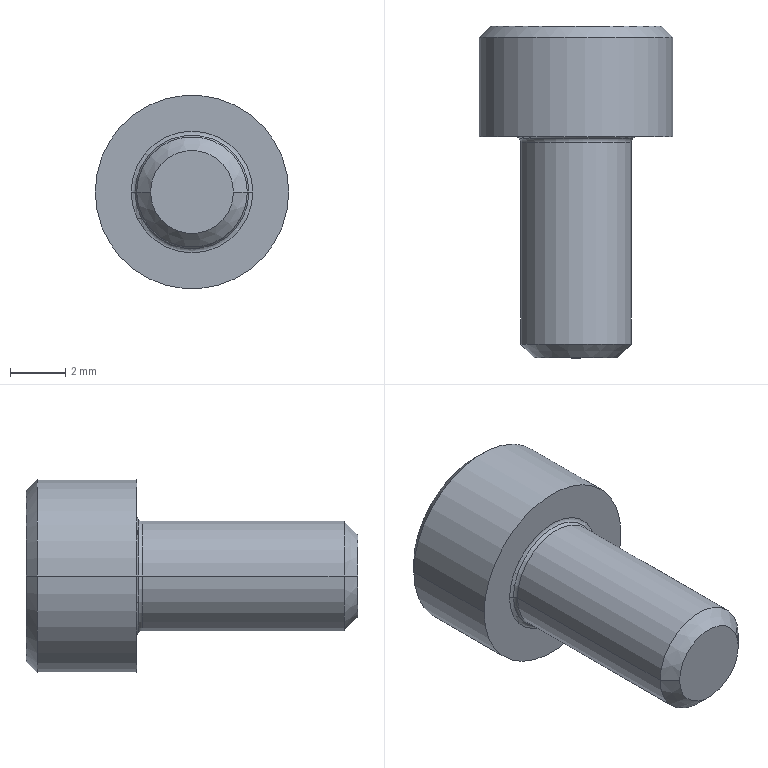Part | Creo | 1 solid | 23 faces | box 7 x 12 x 7 mm | volume 232.803 mm3 | plane 9 | cone 6 | cylinder 4 | torus 4 | commonest cylinder face diameters 4 x2 7 x2
STEP:
#1=CARTESIAN_POINT('',(-77.018,347.995,-340.));
#2=VERTEX_POINT('',#1);
#3=CARTESIAN_POINT('',(-77.884,347.995,-341.5));
#4=VERTEX_POINT('',#3);
#5=CARTESIAN_POINT('',(-77.018,347.995,-340.));
#6=CARTESIAN_POINT('',(-77.058,347.972,-340.07));
#7=CARTESIAN_POINT('',(-77.139,347.93,-340.21));
#8=CARTESIAN_POINT('',(-77.263,347.884,-340.425));
#9=CARTESIAN_POINT('',(-77.389,347.86,-340.642));
#10=CARTESIAN_POINT('',(-77.514,347.86,-340.859));
#11=CARTESIAN_POINT('',(-77.639,347.885,-341.076));
#12=CARTESIAN_POINT('',(-77.763,347.93,-341.291));
#13=CARTESIAN_POINT('',(-77.844,347.972,-341.431));
#14=CARTESIAN_POINT('',(-77.884,347.995,-341.5));
#15=B_SPLINE_CURVE_WITH_KNOTS('',3,(#5,#6,#7,#8,#9,#10,#11,#12,#13,#14),.UNSPECIFIED.,.F.,.F.,(4,1,1,1,1,1,1,4),(0.,0.1429,0.2857,0.4286,0.5714,0.7143,0.8571,1.),.UNSPECIFIED.);
#16=EDGE_CURVE('',#2,#4,#15,.T.);
#17=ORIENTED_EDGE('',*,*,#16,.F.);
#18=CARTESIAN_POINT('',(-78.75,346.995,-340.));
#19=VERTEX_POINT('',#18);
#20=CARTESIAN_POINT('',(-78.75,346.995,-340.));
#21=DIRECTION('',(0.866,0.5,0.));
#22=VECTOR('',#21,2.);
#23=LINE('',#20,#22);
#24=EDGE_CURVE('',#19,#2,#23,.T.);
#25=ORIENTED_EDGE('',*,*,#24,.F.);
#26=CARTESIAN_POINT('',(-80.482,347.995,-340.));
#27=VERTEX_POINT('',#26);
#28=CARTESIAN_POINT('',(-78.75,346.995,-340.));
#29=DIRECTION('',(-0.866,0.5,0.));
#30=VECTOR('',#29,2.);
#31=LINE('',#28,#30);
#32=EDGE_CURVE('',#19,#27,#31,.T.);
#33=ORIENTED_EDGE('',*,*,#32,.T.);
#34=CARTESIAN_POINT('',(-79.616,347.995,-341.5));
#35=VERTEX_POINT('',#34);
#36=CARTESIAN_POINT('',(-79.616,347.995,-341.5));
#37=CARTESIAN_POINT('',(-79.656,347.972,-341.43));
#38=CARTESIAN_POINT('',(-79.737,347.93,-341.29));
#39=CARTESIAN_POINT('',(-79.861,347.884,-341.075));
#40=CARTESIAN_POINT('',(-79.987,347.86,-340.858));
#41=CARTESIAN_POINT('',(-80.112,347.86,-340.641));
#42=CARTESIAN_POINT('',(-80.237,347.885,-340.424));
#43=CARTESIAN_POINT('',(-80.361,347.93,-340.209));
#44=CARTESIAN_POINT('',(-80.442,347.972,-340.069));
#45=CARTESIAN_POINT('',(-80.482,347.995,-340.));
#46=B_SPLINE_CURVE_WITH_KNOTS('',3,(#36,#37,#38,#39,#40,#41,#42,#43,#44,#45),.UNSPECIFIED.,.F.,.F.,(4,1,1,1,1,1,1,4),(0.,0.1429,0.2857,0.4286,0.5714,0.7143,0.8571,1.),.UNSPECIFIED.);
#47=EDGE_CURVE('',#35,#27,#46,.T.);
#48=ORIENTED_EDGE('',*,*,#47,.F.);
#49=CARTESIAN_POINT('',(-77.884,347.995,-341.5));
#50=CARTESIAN_POINT('',(-77.927,347.983,-341.5));
#51=CARTESIAN_POINT('',(-78.013,347.959,-341.5));
#52=CARTESIAN_POINT('',(-78.137,347.93,-341.5));
#53=CARTESIAN_POINT('',(-78.258,347.906,-341.5));
#54=CARTESIAN_POINT('',(-78.379,347.887,-341.5));
#55=CARTESIAN_POINT('',(-78.502,347.872,-341.5));
#56=CARTESIAN_POINT('',(-78.625,347.863,-341.5));
#57=CARTESIAN_POINT('',(-78.75,347.86,-341.5));
#58=CARTESIAN_POINT('',(-78.875,347.863,-341.5));
#59=CARTESIAN_POINT('',(-78.998,347.872,-341.5));
#60=CARTESIAN_POINT('',(-79.121,347.887,-341.5));
#61=CARTESIAN_POINT('',(-79.242,347.906,-341.5));
#62=CARTESIAN_POINT('',(-79.363,347.93,-341.5));
#63=CARTESIAN_POINT('',(-79.487,347.959,-341.5));
#64=CARTESIAN_POINT('',(-79.573,347.983,-341.5));
#65=CARTESIAN_POINT('',(-79.616,347.995,-341.5));
#66=B_SPLINE_CURVE_WITH_KNOTS('',3,(#49,#50,#51,#52,#53,#54,#55,#56,#57,#58,#59,#60,#61,#62,#63,#64,#65),.UNSPECIFIED.,.F.,.F.,(4,1,1,1,1,1,1,1,1,1,1,1,1,1,4),(0.,0.07143,0.1429,0.2143,0.2857,0.3571,0.4286,0.5,0.5714,0.6429,0.7143,0.7857,0.8571,0.9286,1.),.UNSPECIFIED.);
#67=EDGE_CURVE('',#4,#35,#66,.T.);
#68=ORIENTED_EDGE('',*,*,#67,.F.);
#69=EDGE_LOOP('',(#17,#25,#33,#48,#68));
#70=FACE_OUTER_BOUND('',#69,.F.);
#71=CARTESIAN_POINT('',(-78.75,347.505,-340.));
#72=DIRECTION('',(0.,1.,0.));
#73=DIRECTION('',(1.,0.,0.));
#74=AXIS2_PLACEMENT_3D('',#71,#72,#73);
#75=CONICAL_SURFACE('',#74,0.8833,60.);
#76=ADVANCED_FACE('',(#70),#75,.F.);
#77=CARTESIAN_POINT('',(-77.884,349.995,-341.5));
#78=VERTEX_POINT('',#77);
#79=CARTESIAN_POINT('',(-77.018,349.995,-340.));
#80=VERTEX_POINT('',#79);
#81=CARTESIAN_POINT('',(-77.884,349.995,-341.5));
#82=DIRECTION('',(0.5,0.,0.866));
#83=VECTOR('',#82,1.732);
#84=LINE('',#81,#83);
#85=EDGE_CURVE('',#78,#80,#84,.T.);
#86=ORIENTED_EDGE('',*,*,#85,.T.);
#87=CARTESIAN_POINT('',(-77.018,349.995,-340.));
#88=DIRECTION('',(0.,-1.,0.));
#89=VECTOR('',#88,2.);
#90=LINE('',#87,#89);
#91=EDGE_CURVE('',#80,#2,#90,.T.);
#92=ORIENTED_EDGE('',*,*,#91,.T.);
#93=ORIENTED_EDGE('',*,*,#16,.T.);
#94=CARTESIAN_POINT('',(-77.884,349.995,-341.5));
#95=DIRECTION('',(0.,-1.,0.));
#96=VECTOR('',#95,2.);
#97=LINE('',#94,#96);
#98=EDGE_CURVE('',#78,#4,#97,.T.);
#99=ORIENTED_EDGE('',*,*,#98,.F.);
#100=EDGE_LOOP('',(#86,#92,#93,#99));
#101=FACE_OUTER_BOUND('',#100,.F.);
#102=CARTESIAN_POINT('',(-77.884,347.995,-341.5));
#103=DIRECTION('',(-0.866,0.,0.5));
#104=DIRECTION('',(0.5,0.,0.866));
#105=AXIS2_PLACEMENT_3D('',#102,#103,#104);
#106=PLANE('',#105);
#107=ADVANCED_FACE('',(#101),#106,.T.);
#108=CARTESIAN_POINT('',(-75.65,349.995,-340.));
#109=VERTEX_POINT('',#108);
#110=CARTESIAN_POINT('',(-81.85,349.995,-340.));
#111=VERTEX_POINT('',#110);
#112=CARTESIAN_POINT('',(-78.75,349.995,-340.));
#113=DIRECTION('',(0.,1.,0.));
#114=DIRECTION('',(1.,0.,0.));
#115=AXIS2_PLACEMENT_3D('',#112,#113,#114);
#116=CIRCLE('',#115,3.1);
#117=EDGE_CURVE('',#109,#111,#116,.T.);
#118=ORIENTED_EDGE('',*,*,#117,.F.);
#119=CARTESIAN_POINT('',(-78.75,349.995,-340.));
#120=DIRECTION('',(0.,1.,0.));
#121=DIRECTION('',(-1.,0.,0.));
#122=AXIS2_PLACEMENT_3D('',#119,#120,#121);
#123=CIRCLE('',#122,3.1);
#124=EDGE_CURVE('',#111,#109,#123,.T.);
#125=ORIENTED_EDGE('',*,*,#124,.F.);
#126=EDGE_LOOP('',(#118,#125));
#127=FACE_OUTER_BOUND('',#126,.F.);
#128=CARTESIAN_POINT('',(-77.884,349.995,-338.5));
#129=VERTEX_POINT('',#128);
#130=CARTESIAN_POINT('',(-77.018,349.995,-340.));
#131=DIRECTION('',(-0.5,0.,0.866));
#132=VECTOR('',#131,1.732);
#133=LINE('',#130,#132);
#134=EDGE_CURVE('',#80,#129,#133,.T.);
#135=ORIENTED_EDGE('',*,*,#134,.F.);
#136=ORIENTED_EDGE('',*,*,#85,.F.);
#137=CARTESIAN_POINT('',(-79.616,349.995,-341.5));
#138=VERTEX_POINT('',#137);
#139=CARTESIAN_POINT('',(-77.884,349.995,-341.5));
#140=DIRECTION('',(-1.,0.,0.));
#141=VECTOR('',#140,1.732);
#142=LINE('',#139,#141);
#143=EDGE_CURVE('',#78,#138,#142,.T.);
#144=ORIENTED_EDGE('',*,*,#143,.T.);
#145=CARTESIAN_POINT('',(-80.482,349.995,-340.));
#146=VERTEX_POINT('',#145);
#147=CARTESIAN_POINT('',(-80.482,349.995,-340.));
#148=DIRECTION('',(0.5,0.,-0.866));
#149=VECTOR('',#148,1.732);
#150=LINE('',#147,#149);
#151=EDGE_CURVE('',#146,#138,#150,.T.);
#152=ORIENTED_EDGE('',*,*,#151,.F.);
#153=CARTESIAN_POINT('',(-79.616,349.995,-338.5));
#154=VERTEX_POINT('',#153);
#155=CARTESIAN_POINT('',(-79.616,349.995,-338.5));
#156=DIRECTION('',(-0.5,0.,-0.866));
#157=VECTOR('',#156,1.732);
#158=LINE('',#155,#157);
#159=EDGE_CURVE('',#154,#146,#158,.T.);
#160=ORIENTED_EDGE('',*,*,#159,.F.);
#161=CARTESIAN_POINT('',(-79.616,349.995,-338.5));
#162=DIRECTION('',(1.,0.,0.));
#163=VECTOR('',#162,1.732);
#164=LINE('',#161,#163);
#165=EDGE_CURVE('',#154,#129,#164,.T.);
#166=ORIENTED_EDGE('',*,*,#165,.T.);
#167=EDGE_LOOP('',(#135,#136,#144,#152,#160,#166));
#168=FACE_BOUND('',#167,.F.);
#169=CARTESIAN_POINT('',(-78.75,349.995,-340.));
#170=DIRECTION('',(0.,1.,0.));
#171=DIRECTION('',(1.,0.,0.));
#172=AXIS2_PLACEMENT_3D('',#169,#170,#171);
#173=PLANE('',#172);
#174=ADVANCED_FACE('',(#127,#168),#173,.T.);
#175=CARTESIAN_POINT('',(-75.25,349.595,-340.));
#176=VERTEX_POINT('',#175);
#177=CARTESIAN_POINT('',(-82.25,349.595,-340.));
#178=VERTEX_POINT('',#177);
#179=CARTESIAN_POINT('',(-78.75,349.595,-340.));
#180=DIRECTION('',(0.,1.,0.));
#181=DIRECTION('',(1.,0.,0.));
#182=AXIS2_PLACEMENT_3D('',#179,#180,#181);
#183=CIRCLE('',#182,3.5);
#184=EDGE_CURVE('',#176,#178,#183,.T.);
#185=ORIENTED_EDGE('',*,*,#184,.F.);
#186=CARTESIAN_POINT('',(-75.65,349.995,-340.));
#187=DIRECTION('',(0.7071,-0.7071,0.));
#188=VECTOR('',#187,0.5657);
#189=LINE('',#186,#188);
#190=EDGE_CURVE('',#109,#176,#189,.T.);
#191=ORIENTED_EDGE('',*,*,#190,.F.);
#192=ORIENTED_EDGE('',*,*,#117,.T.);
#193=CARTESIAN_POINT('',(-81.85,349.995,-340.));
#194=DIRECTION('',(-0.7071,-0.7071,0.));
#195=VECTOR('',#194,0.5657);
#196=LINE('',#193,#195);
#197=EDGE_CURVE('',#111,#178,#196,.T.);
#198=ORIENTED_EDGE('',*,*,#197,.T.);
#199=EDGE_LOOP('',(#185,#191,#192,#198));
#200=FACE_OUTER_BOUND('',#199,.F.);
#201=CARTESIAN_POINT('',(-78.75,349.795,-340.));
#202=DIRECTION('',(0.,-1.,0.));
#203=DIRECTION('',(-1.,0.,0.));
#204=AXIS2_PLACEMENT_3D('',#201,#202,#203);
#205=CONICAL_SURFACE('',#204,3.3,45.);
#206=ADVANCED_FACE('',(#200),#205,.T.);
#207=ORIENTED_EDGE('',*,*,#184,.T.);
#208=CARTESIAN_POINT('',(-82.25,345.995,-340.));
#209=VERTEX_POINT('',#208);
#210=CARTESIAN_POINT('',(-82.25,345.995,-340.));
#211=DIRECTION('',(0.,1.,0.));
#212=VECTOR('',#211,3.6);
#213=LINE('',#210,#212);
#214=EDGE_CURVE('',#209,#178,#213,.T.);
#215=ORIENTED_EDGE('',*,*,#214,.F.);
#216=CARTESIAN_POINT('',(-75.25,345.995,-340.));
#217=VERTEX_POINT('',#216);
#218=CARTESIAN_POINT('',(-78.75,345.995,-340.));
#219=DIRECTION('',(0.,-1.,0.));
#220=DIRECTION('',(-1.,0.,0.));
#221=AXIS2_PLACEMENT_3D('',#218,#219,#220);
#222=CIRCLE('',#221,3.5);
#223=EDGE_CURVE('',#209,#217,#222,.T.);
#224=ORIENTED_EDGE('',*,*,#223,.T.);
#225=CARTESIAN_POINT('',(-75.25,345.995,-340.));
#226=DIRECTION('',(0.,1.,0.));
#227=VECTOR('',#226,3.6);
#228=LINE('',#225,#227);
#229=EDGE_CURVE('',#217,#176,#228,.T.);
#230=ORIENTED_EDGE('',*,*,#229,.T.);
#231=EDGE_LOOP('',(#207,#215,#224,#230));
#232=FACE_OUTER_BOUND('',#231,.F.);
#233=CARTESIAN_POINT('',(-78.75,345.995,-340.));
#234=DIRECTION('',(0.,1.,0.));
#235=DIRECTION('',(1.,0.,0.));
#236=AXIS2_PLACEMENT_3D('',#233,#234,#235);
#237=CYLINDRICAL_SURFACE('',#236,3.5);
#238=ADVANCED_FACE('',(#232),#237,.T.);
#239=CARTESIAN_POINT('',(-78.75,349.595,-340.));
#240=DIRECTION('',(0.,1.,0.));
#241=DIRECTION('',(-1.,0.,0.));
#242=AXIS2_PLACEMENT_3D('',#239,#240,#241);
#243=CIRCLE('',#242,3.5);
#244=EDGE_CURVE('',#178,#176,#243,.T.);
#245=ORIENTED_EDGE('',*,*,#244,.T.);
#246=ORIENTED_EDGE('',*,*,#229,.F.);
#247=CARTESIAN_POINT('',(-78.75,345.995,-340.));
#248=DIRECTION('',(0.,-1.,0.));
#249=DIRECTION('',(1.,0.,0.));
#250=AXIS2_PLACEMENT_3D('',#247,#248,#249);
#251=CIRCLE('',#250,3.5);
#252=EDGE_CURVE('',#217,#209,#251,.T.);
#253=ORIENTED_EDGE('',*,*,#252,.T.);
#254=ORIENTED_EDGE('',*,*,#214,.T.);
#255=EDGE_LOOP('',(#245,#246,#253,#254));
#256=FACE_OUTER_BOUND('',#255,.F.);
#257=CARTESIAN_POINT('',(-78.75,345.995,-340.));
#258=DIRECTION('',(0.,1.,0.));
#259=DIRECTION('',(1.,0.,0.));
#260=AXIS2_PLACEMENT_3D('',#257,#258,#259);
#261=CYLINDRICAL_SURFACE('',#260,3.5);
#262=ADVANCED_FACE('',(#256),#261,.T.);
#263=ORIENTED_EDGE('',*,*,#244,.F.);
#264=ORIENTED_EDGE('',*,*,#197,.F.);
#265=ORIENTED_EDGE('',*,*,#124,.T.);
#266=ORIENTED_EDGE('',*,*,#190,.T.);
#267=EDGE_LOOP('',(#263,#264,#265,#266));
#268=FACE_OUTER_BOUND('',#267,.F.);
#269=CARTESIAN_POINT('',(-78.75,349.795,-340.));
#270=DIRECTION('',(0.,-1.,0.));
#271=DIRECTION('',(-1.,0.,0.));
#272=AXIS2_PLACEMENT_3D('',#269,#270,#271);
#273=CONICAL_SURFACE('',#272,3.3,45.);
#274=ADVANCED_FACE('',(#268),#273,.T.);
#275=ORIENTED_EDGE('',*,*,#252,.F.);
#276=ORIENTED_EDGE('',*,*,#223,.F.);
#277=EDGE_LOOP('',(#275,#276));
#278=FACE_OUTER_BOUND('',#277,.F.);
#279=CARTESIAN_POINT('',(-76.55,345.995,-340.));
#280=VERTEX_POINT('',#279);
#281=CARTESIAN_POINT('',(-80.95,345.995,-340.));
#282=VERTEX_POINT('',#281);
#283=CARTESIAN_POINT('',(-78.75,345.995,-340.));
#284=DIRECTION('',(0.,1.,0.));
#285=DIRECTION('',(1.,0.,0.));
#286=AXIS2_PLACEMENT_3D('',#283,#284,#285);
#287=CIRCLE('',#286,2.2);
#288=EDGE_CURVE('',#280,#282,#287,.T.);
#289=ORIENTED_EDGE('',*,*,#288,.F.);
#290=CARTESIAN_POINT('',(-78.75,345.995,-340.));
#291=DIRECTION('',(0.,1.,0.));
#292=DIRECTION('',(-1.,0.,0.));
#293=AXIS2_PLACEMENT_3D('',#290,#291,#292);
#294=CIRCLE('',#293,2.2);
#295=EDGE_CURVE('',#282,#280,#294,.T.);
#296=ORIENTED_EDGE('',*,*,#295,.F.);
#297=EDGE_LOOP('',(#289,#296));
#298=FACE_BOUND('',#297,.F.);
#299=CARTESIAN_POINT('',(-78.75,345.995,-340.));
#300=DIRECTION('',(0.,1.,0.));
#301=DIRECTION('',(1.,0.,0.));
#302=AXIS2_PLACEMENT_3D('',#299,#300,#301);
#303=PLANE('',#302);
#304=ADVANCED_FACE('',(#278,#298),#303,.F.);
#305=ORIENTED_EDGE('',*,*,#288,.T.);
#306=CARTESIAN_POINT('',(-80.809,345.937,-340.));
#307=VERTEX_POINT('',#306);
#308=CARTESIAN_POINT('',(-80.95,345.795,-340.));
#309=DIRECTION('',(0.,0.,-1.));
#310=DIRECTION('',(0.,1.,0.));
#311=AXIS2_PLACEMENT_3D('',#308,#309,#310);
#312=CIRCLE('',#311,0.2);
#313=EDGE_CURVE('',#282,#307,#312,.T.);
#314=ORIENTED_EDGE('',*,*,#313,.T.);
#315=CARTESIAN_POINT('',(-76.691,345.937,-340.));
#316=VERTEX_POINT('',#315);
#317=CARTESIAN_POINT('',(-78.75,345.937,-340.));
#318=DIRECTION('',(0.,1.,0.));
#319=DIRECTION('',(1.,0.,0.));
#320=AXIS2_PLACEMENT_3D('',#317,#318,#319);
#321=CIRCLE('',#320,2.059);
#322=EDGE_CURVE('',#316,#307,#321,.T.);
#323=ORIENTED_EDGE('',*,*,#322,.F.);
#324=CARTESIAN_POINT('',(-76.55,345.795,-340.));
#325=DIRECTION('',(0.,0.,1.));
#326=DIRECTION('',(0.,1.,0.));
#327=AXIS2_PLACEMENT_3D('',#324,#325,#326);
#328=CIRCLE('',#327,0.2);
#329=EDGE_CURVE('',#280,#316,#328,.T.);
#330=ORIENTED_EDGE('',*,*,#329,.F.);
#331=EDGE_LOOP('',(#305,#314,#323,#330));
#332=FACE_OUTER_BOUND('',#331,.F.);
#333=CARTESIAN_POINT('',(-78.75,345.795,-340.));
#334=DIRECTION('',(0.,1.,0.));
#335=DIRECTION('',(1.,0.,0.));
#336=AXIS2_PLACEMENT_3D('',#333,#334,#335);
#337=TOROIDAL_SURFACE('',#336,2.2,0.2);
#338=ADVANCED_FACE('',(#332),#337,.F.);
#339=ORIENTED_EDGE('',*,*,#295,.T.);
#340=ORIENTED_EDGE('',*,*,#329,.T.);
#341=CARTESIAN_POINT('',(-78.75,345.937,-340.));
#342=DIRECTION('',(0.,1.,0.));
#343=DIRECTION('',(-1.,0.,0.));
#344=AXIS2_PLACEMENT_3D('',#341,#342,#343);
#345=CIRCLE('',#344,2.059);
#346=EDGE_CURVE('',#307,#316,#345,.T.);
#347=ORIENTED_EDGE('',*,*,#346,.F.);
#348=ORIENTED_EDGE('',*,*,#313,.F.);
#349=EDGE_LOOP('',(#339,#340,#347,#348));
#350=FACE_OUTER_BOUND('',#349,.F.);
#351=CARTESIAN_POINT('',(-78.75,345.795,-340.));
#352=DIRECTION('',(0.,1.,0.));
#353=DIRECTION('',(1.,0.,0.));
#354=AXIS2_PLACEMENT_3D('',#351,#352,#353);
#355=TOROIDAL_SURFACE('',#354,2.2,0.2);
#356=ADVANCED_FACE('',(#350),#355,.F.);
#357=CARTESIAN_POINT('',(-80.75,345.795,-340.));
#358=VERTEX_POINT('',#357);
#359=CARTESIAN_POINT('',(-76.75,345.795,-340.));
#360=VERTEX_POINT('',#359);
#361=CARTESIAN_POINT('',(-78.75,345.795,-340.));
#362=DIRECTION('',(0.,1.,0.));
#363=DIRECTION('',(-1.,0.,0.));
#364=AXIS2_PLACEMENT_3D('',#361,#362,#363);
#365=CIRCLE('',#364,2.);
#366=EDGE_CURVE('',#358,#360,#365,.T.);
#367=ORIENTED_EDGE('',*,*,#366,.F.);
#368=CARTESIAN_POINT('',(-80.95,345.795,-340.));
#369=DIRECTION('',(0.,0.,-1.));
#370=DIRECTION('',(0.7071,0.7071,0.));
#371=AXIS2_PLACEMENT_3D('',#368,#369,#370);
#372=CIRCLE('',#371,0.2);
#373=EDGE_CURVE('',#307,#358,#372,.T.);
#374=ORIENTED_EDGE('',*,*,#373,.F.);
#375=ORIENTED_EDGE('',*,*,#346,.T.);
#376=CARTESIAN_POINT('',(-76.55,345.795,-340.));
#377=DIRECTION('',(0.,0.,1.));
#378=DIRECTION('',(-0.7071,0.7071,0.));
#379=AXIS2_PLACEMENT_3D('',#376,#377,#378);
#380=CIRCLE('',#379,0.2);
#381=EDGE_CURVE('',#316,#360,#380,.T.);
#382=ORIENTED_EDGE('',*,*,#381,.T.);
#383=EDGE_LOOP('',(#367,#374,#375,#382));
#384=FACE_OUTER_BOUND('',#383,.F.);
#385=CARTESIAN_POINT('',(-78.75,345.795,-340.));
#386=DIRECTION('',(0.,1.,0.));
#387=DIRECTION('',(1.,0.,0.));
#388=AXIS2_PLACEMENT_3D('',#385,#386,#387);
#389=TOROIDAL_SURFACE('',#388,2.2,0.2);
#390=ADVANCED_FACE('',(#384),#389,.F.);
#391=CARTESIAN_POINT('',(-76.75,338.495,-340.));
#392=VERTEX_POINT('',#391);
#393=CARTESIAN_POINT('',(-80.75,338.495,-340.));
#394=VERTEX_POINT('',#393);
#395=CARTESIAN_POINT('',(-78.75,338.495,-340.));
#396=DIRECTION('',(0.,-1.,0.));
#397=DIRECTION('',(1.,0.,0.));
#398=AXIS2_PLACEMENT_3D('',#395,#396,#397);
#399=CIRCLE('',#398,2.);
#400=EDGE_CURVE('',#392,#394,#399,.T.);
#401=ORIENTED_EDGE('',*,*,#400,.T.);
#402=CARTESIAN_POINT('',(-80.75,338.495,-340.));
#403=DIRECTION('',(0.,1.,0.));
#404=VECTOR('',#403,7.3);
#405=LINE('',#402,#404);
#406=EDGE_CURVE('',#394,#358,#405,.T.);
#407=ORIENTED_EDGE('',*,*,#406,.T.);
#408=ORIENTED_EDGE('',*,*,#366,.T.);
#409=CARTESIAN_POINT('',(-76.75,338.495,-340.));
#410=DIRECTION('',(0.,1.,0.));
#411=VECTOR('',#410,7.3);
#412=LINE('',#409,#411);
#413=EDGE_CURVE('',#392,#360,#412,.T.);
#414=ORIENTED_EDGE('',*,*,#413,.F.);
#415=EDGE_LOOP('',(#401,#407,#408,#414));
#416=FACE_OUTER_BOUND('',#415,.F.);
#417=CARTESIAN_POINT('',(-78.75,337.995,-340.));
#418=DIRECTION('',(0.,1.,0.));
#419=DIRECTION('',(1.,0.,0.));
#420=AXIS2_PLACEMENT_3D('',#417,#418,#419);
#421=CYLINDRICAL_SURFACE('',#420,2.);
#422=ADVANCED_FACE('',(#416),#421,.T.);
#423=CARTESIAN_POINT('',(-77.25,337.995,-340.));
#424=VERTEX_POINT('',#423);
#425=CARTESIAN_POINT('',(-80.25,337.995,-340.));
#426=VERTEX_POINT('',#425);
#427=CARTESIAN_POINT('',(-78.75,337.995,-340.));
#428=DIRECTION('',(0.,-1.,0.));
#429=DIRECTION('',(1.,0.,0.));
#430=AXIS2_PLACEMENT_3D('',#427,#428,#429);
#431=CIRCLE('',#430,1.5);
#432=EDGE_CURVE('',#424,#426,#431,.T.);
#433=ORIENTED_EDGE('',*,*,#432,.T.);
#434=CARTESIAN_POINT('',(-80.25,337.995,-340.));
#435=DIRECTION('',(-0.7071,0.7071,0.));
#436=VECTOR('',#435,0.7071);
#437=LINE('',#434,#436);
#438=EDGE_CURVE('',#426,#394,#437,.T.);
#439=ORIENTED_EDGE('',*,*,#438,.T.);
#440=ORIENTED_EDGE('',*,*,#400,.F.);
#441=CARTESIAN_POINT('',(-77.25,337.995,-340.));
#442=DIRECTION('',(0.7071,0.7071,0.));
#443=VECTOR('',#442,0.7071);
#444=LINE('',#441,#443);
#445=EDGE_CURVE('',#424,#392,#444,.T.);
#446=ORIENTED_EDGE('',*,*,#445,.F.);
#447=EDGE_LOOP('',(#433,#439,#440,#446));
#448=FACE_OUTER_BOUND('',#447,.F.);
#449=CARTESIAN_POINT('',(-78.75,338.245,-340.));
#450=DIRECTION('',(0.,1.,0.));
#451=DIRECTION('',(1.,0.,0.));
#452=AXIS2_PLACEMENT_3D('',#449,#450,#451);
#453=CONICAL_SURFACE('',#452,1.75,45.);
#454=ADVANCED_FACE('',(#448),#453,.T.);
#455=ORIENTED_EDGE('',*,*,#432,.F.);
#456=CARTESIAN_POINT('',(-78.75,337.995,-340.));
#457=DIRECTION('',(0.,-1.,0.));
#458=DIRECTION('',(-1.,0.,0.));
#459=AXIS2_PLACEMENT_3D('',#456,#457,#458);
#460=CIRCLE('',#459,1.5);
#461=EDGE_CURVE('',#426,#424,#460,.T.);
#462=ORIENTED_EDGE('',*,*,#461,.F.);
#463=EDGE_LOOP('',(#455,#462));
#464=FACE_OUTER_BOUND('',#463,.F.);
#465=CARTESIAN_POINT('',(-78.75,337.995,-340.));
#466=DIRECTION('',(0.,1.,0.));
#467=DIRECTION('',(1.,0.,0.));
#468=AXIS2_PLACEMENT_3D('',#465,#466,#467);
#469=PLANE('',#468);
#470=ADVANCED_FACE('',(#464),#469,.F.);
#471=ORIENTED_EDGE('',*,*,#461,.T.);
#472=ORIENTED_EDGE('',*,*,#445,.T.);
#473=CARTESIAN_POINT('',(-78.75,338.495,-340.));
#474=DIRECTION('',(0.,-1.,0.));
#475=DIRECTION('',(-1.,0.,0.));
#476=AXIS2_PLACEMENT_3D('',#473,#474,#475);
#477=CIRCLE('',#476,2.);
#478=EDGE_CURVE('',#394,#392,#477,.T.);
#479=ORIENTED_EDGE('',*,*,#478,.F.);
#480=ORIENTED_EDGE('',*,*,#438,.F.);
#481=EDGE_LOOP('',(#471,#472,#479,#480));
#482=FACE_OUTER_BOUND('',#481,.F.);
#483=CARTESIAN_POINT('',(-78.75,338.245,-340.));
#484=DIRECTION('',(0.,1.,0.));
#485=DIRECTION('',(1.,0.,0.));
#486=AXIS2_PLACEMENT_3D('',#483,#484,#485);
#487=CONICAL_SURFACE('',#486,1.75,45.);
#488=ADVANCED_FACE('',(#482),#487,.T.);
#489=ORIENTED_EDGE('',*,*,#478,.T.);
#490=ORIENTED_EDGE('',*,*,#413,.T.);
#491=CARTESIAN_POINT('',(-78.75,345.795,-340.));
#492=DIRECTION('',(0.,1.,0.));
#493=DIRECTION('',(1.,0.,0.));
#494=AXIS2_PLACEMENT_3D('',#491,#492,#493);
#495=CIRCLE('',#494,2.);
#496=EDGE_CURVE('',#360,#358,#495,.T.);
#497=ORIENTED_EDGE('',*,*,#496,.T.);
#498=ORIENTED_EDGE('',*,*,#406,.F.);
#499=EDGE_LOOP('',(#489,#490,#497,#498));
#500=FACE_OUTER_BOUND('',#499,.F.);
#501=CARTESIAN_POINT('',(-78.75,337.995,-340.));
#502=DIRECTION('',(0.,1.,0.));
#503=DIRECTION('',(1.,0.,0.));
#504=AXIS2_PLACEMENT_3D('',#501,#502,#503);
#505=CYLINDRICAL_SURFACE('',#504,2.);
#506=ADVANCED_FACE('',(#500),#505,.T.);
#507=ORIENTED_EDGE('',*,*,#496,.F.);
#508=ORIENTED_EDGE('',*,*,#381,.F.);
#509=ORIENTED_EDGE('',*,*,#322,.T.);
#510=ORIENTED_EDGE('',*,*,#373,.T.);
#511=EDGE_LOOP('',(#507,#508,#509,#510));
#512=FACE_OUTER_BOUND('',#511,.F.);
#513=CARTESIAN_POINT('',(-78.75,345.795,-340.));
#514=DIRECTION('',(0.,1.,0.));
#515=DIRECTION('',(1.,0.,0.));
#516=AXIS2_PLACEMENT_3D('',#513,#514,#515);
#517=TOROIDAL_SURFACE('',#516,2.2,0.2);
#518=ADVANCED_FACE('',(#512),#517,.F.);
#519=ORIENTED_EDGE('',*,*,#134,.T.);
#520=CARTESIAN_POINT('',(-77.884,347.995,-338.5));
#521=VERTEX_POINT('',#520);
#522=CARTESIAN_POINT('',(-77.884,349.995,-338.5));
#523=DIRECTION('',(0.,-1.,0.));
#524=VECTOR('',#523,2.);
#525=LINE('',#522,#524);
#526=EDGE_CURVE('',#129,#521,#525,.T.);
#527=ORIENTED_EDGE('',*,*,#526,.T.);
#528=CARTESIAN_POINT('',(-77.884,347.995,-338.5));
#529=CARTESIAN_POINT('',(-77.844,347.972,-338.57));
#530=CARTESIAN_POINT('',(-77.763,347.93,-338.71));
#531=CARTESIAN_POINT('',(-77.639,347.884,-338.925));
#532=CARTESIAN_POINT('',(-77.513,347.86,-339.142));
#533=CARTESIAN_POINT('',(-77.388,347.86,-339.359));
#534=CARTESIAN_POINT('',(-77.263,347.885,-339.576));
#535=CARTESIAN_POINT('',(-77.139,347.93,-339.791));
#536=CARTESIAN_POINT('',(-77.058,347.972,-339.931));
#537=CARTESIAN_POINT('',(-77.018,347.995,-340.));
#538=B_SPLINE_CURVE_WITH_KNOTS('',3,(#528,#529,#530,#531,#532,#533,#534,#535,#536,#537),.UNSPECIFIED.,.F.,.F.,(4,1,1,1,1,1,1,4),(0.,0.1429,0.2857,0.4286,0.5714,0.7143,0.8571,1.),.UNSPECIFIED.);
#539=EDGE_CURVE('',#521,#2,#538,.T.);
#540=ORIENTED_EDGE('',*,*,#539,.T.);
#541=ORIENTED_EDGE('',*,*,#91,.F.);
#542=EDGE_LOOP('',(#519,#527,#540,#541));
#543=FACE_OUTER_BOUND('',#542,.F.);
#544=CARTESIAN_POINT('',(-77.018,347.995,-340.));
#545=DIRECTION('',(-0.866,0.,-0.5));
#546=DIRECTION('',(-0.5,0.,0.866));
#547=AXIS2_PLACEMENT_3D('',#544,#545,#546);
#548=PLANE('',#547);
#549=ADVANCED_FACE('',(#543),#548,.T.);
#550=ORIENTED_EDGE('',*,*,#165,.F.);
#551=CARTESIAN_POINT('',(-79.616,347.995,-338.5));
#552=VERTEX_POINT('',#551);
#553=CARTESIAN_POINT('',(-79.616,349.995,-338.5));
#554=DIRECTION('',(0.,-1.,0.));
#555=VECTOR('',#554,2.);
#556=LINE('',#553,#555);
#557=EDGE_CURVE('',#154,#552,#556,.T.);
#558=ORIENTED_EDGE('',*,*,#557,.T.);
#559=CARTESIAN_POINT('',(-79.616,347.995,-338.5));
#560=CARTESIAN_POINT('',(-79.573,347.983,-338.5));
#561=CARTESIAN_POINT('',(-79.487,347.959,-338.5));
#562=CARTESIAN_POINT('',(-79.363,347.93,-338.5));
#563=CARTESIAN_POINT('',(-79.242,347.906,-338.5));
#564=CARTESIAN_POINT('',(-79.121,347.887,-338.5));
#565=CARTESIAN_POINT('',(-78.998,347.872,-338.5));
#566=CARTESIAN_POINT('',(-78.875,347.863,-338.5));
#567=CARTESIAN_POINT('',(-78.75,347.86,-338.5));
#568=CARTESIAN_POINT('',(-78.625,347.863,-338.5));
#569=CARTESIAN_POINT('',(-78.502,347.872,-338.5));
#570=CARTESIAN_POINT('',(-78.379,347.887,-338.5));
#571=CARTESIAN_POINT('',(-78.258,347.906,-338.5));
#572=CARTESIAN_POINT('',(-78.137,347.93,-338.5));
#573=CARTESIAN_POINT('',(-78.013,347.959,-338.5));
#574=CARTESIAN_POINT('',(-77.927,347.983,-338.5));
#575=CARTESIAN_POINT('',(-77.884,347.995,-338.5));
#576=B_SPLINE_CURVE_WITH_KNOTS('',3,(#559,#560,#561,#562,#563,#564,#565,#566,#567,#568,#569,#570,#571,#572,#573,#574,#575),.UNSPECIFIED.,.F.,.F.,(4,1,1,1,1,1,1,1,1,1,1,1,1,1,4),(0.,0.07143,0.1429,0.2143,0.2857,0.3571,0.4286,0.5,0.5714,0.6429,0.7143,0.7857,0.8571,0.9286,1.),.UNSPECIFIED.);
#577=EDGE_CURVE('',#552,#521,#576,.T.);
#578=ORIENTED_EDGE('',*,*,#577,.T.);
#579=ORIENTED_EDGE('',*,*,#526,.F.);
#580=EDGE_LOOP('',(#550,#558,#578,#579));
#581=FACE_OUTER_BOUND('',#580,.F.);
#582=CARTESIAN_POINT('',(-77.884,347.995,-338.5));
#583=DIRECTION('',(0.,0.,-1.));
#584=DIRECTION('',(0.,1.,0.));
#585=AXIS2_PLACEMENT_3D('',#582,#583,#584);
#586=PLANE('',#585);
#587=ADVANCED_FACE('',(#581),#586,.T.);
#588=ORIENTED_EDGE('',*,*,#159,.T.);
#589=CARTESIAN_POINT('',(-80.482,349.995,-340.));
#590=DIRECTION('',(0.,-1.,0.));
#591=VECTOR('',#590,2.);
#592=LINE('',#589,#591);
#593=EDGE_CURVE('',#146,#27,#592,.T.);
#594=ORIENTED_EDGE('',*,*,#593,.T.);
#595=CARTESIAN_POINT('',(-80.482,347.995,-340.));
#596=CARTESIAN_POINT('',(-80.442,347.972,-339.931));
#597=CARTESIAN_POINT('',(-80.361,347.93,-339.791));
#598=CARTESIAN_POINT('',(-80.237,347.885,-339.576));
#599=CARTESIAN_POINT('',(-80.112,347.86,-339.359));
#600=CARTESIAN_POINT('',(-79.987,347.86,-339.142));
#601=CARTESIAN_POINT('',(-79.861,347.884,-338.925));
#602=CARTESIAN_POINT('',(-79.737,347.93,-338.71));
#603=CARTESIAN_POINT('',(-79.656,347.972,-338.57));
#604=CARTESIAN_POINT('',(-79.616,347.995,-338.5));
#605=B_SPLINE_CURVE_WITH_KNOTS('',3,(#595,#596,#597,#598,#599,#600,#601,#602,#603,#604),.UNSPECIFIED.,.F.,.F.,(4,1,1,1,1,1,1,4),(0.,0.1429,0.2857,0.4286,0.5714,0.7143,0.8571,1.),.UNSPECIFIED.);
#606=EDGE_CURVE('',#27,#552,#605,.T.);
#607=ORIENTED_EDGE('',*,*,#606,.T.);
#608=ORIENTED_EDGE('',*,*,#557,.F.);
#609=EDGE_LOOP('',(#588,#594,#607,#608));
#610=FACE_OUTER_BOUND('',#609,.F.);
#611=CARTESIAN_POINT('',(-79.616,347.995,-338.5));
#612=DIRECTION('',(0.866,0.,-0.5));
#613=DIRECTION('',(-0.5,0.,-0.866));
#614=AXIS2_PLACEMENT_3D('',#611,#612,#613);
#615=PLANE('',#614);
#616=ADVANCED_FACE('',(#610),#615,.T.);
#617=ORIENTED_EDGE('',*,*,#151,.T.);
#618=CARTESIAN_POINT('',(-79.616,349.995,-341.5));
#619=DIRECTION('',(0.,-1.,0.));
#620=VECTOR('',#619,2.);
#621=LINE('',#618,#620);
#622=EDGE_CURVE('',#138,#35,#621,.T.);
#623=ORIENTED_EDGE('',*,*,#622,.T.);
#624=ORIENTED_EDGE('',*,*,#47,.T.);
#625=ORIENTED_EDGE('',*,*,#593,.F.);
#626=EDGE_LOOP('',(#617,#623,#624,#625));
#627=FACE_OUTER_BOUND('',#626,.F.);
#628=CARTESIAN_POINT('',(-80.482,347.995,-340.));
#629=DIRECTION('',(0.866,0.,0.5));
#630=DIRECTION('',(0.5,0.,-0.866));
#631=AXIS2_PLACEMENT_3D('',#628,#629,#630);
#632=PLANE('',#631);
#633=ADVANCED_FACE('',(#627),#632,.T.);
#634=ORIENTED_EDGE('',*,*,#143,.F.);
#635=ORIENTED_EDGE('',*,*,#98,.T.);
#636=ORIENTED_EDGE('',*,*,#67,.T.);
#637=ORIENTED_EDGE('',*,*,#622,.F.);
#638=EDGE_LOOP('',(#634,#635,#636,#637));
#639=FACE_OUTER_BOUND('',#638,.F.);
#640=CARTESIAN_POINT('',(-79.616,347.995,-341.5));
#641=DIRECTION('',(0.,0.,1.));
#642=DIRECTION('',(0.,-1.,0.));
#643=AXIS2_PLACEMENT_3D('',#640,#641,#642);
#644=PLANE('',#643);
#645=ADVANCED_FACE('',(#639),#644,.T.);
#646=ORIENTED_EDGE('',*,*,#606,.F.);
#647=ORIENTED_EDGE('',*,*,#32,.F.);
#648=ORIENTED_EDGE('',*,*,#24,.T.);
#649=ORIENTED_EDGE('',*,*,#539,.F.);
#650=ORIENTED_EDGE('',*,*,#577,.F.);
#651=EDGE_LOOP('',(#646,#647,#648,#649,#650));
#652=FACE_OUTER_BOUND('',#651,.F.);
#653=CARTESIAN_POINT('',(-78.75,347.505,-340.));
#654=DIRECTION('',(0.,1.,0.));
#655=DIRECTION('',(1.,0.,0.));
#656=AXIS2_PLACEMENT_3D('',#653,#654,#655);
#657=CONICAL_SURFACE('',#656,0.8833,60.);
#658=ADVANCED_FACE('',(#652),#657,.F.);
#659=CLOSED_SHELL('',(#76,#107,#174,#206,#238,#262,#274,#304,#338,#356,#390,#422,#454,#470,#488,#506,#518,#549,#587,#616,#633,#645,#658));
#660=MANIFOLD_SOLID_BREP('',#659);
#661=(LENGTH_UNIT()NAMED_UNIT(*)SI_UNIT(.MILLI.,.METRE.));
#662=UNCERTAINTY_MEASURE_WITH_UNIT(LENGTH_MEASURE(0.001556),#661,'','');
#663=(NAMED_UNIT(*)PLANE_ANGLE_UNIT()SI_UNIT($,.RADIAN.));
#664=PLANE_ANGLE_MEASURE_WITH_UNIT(PLANE_ANGLE_MEASURE(0.01745),#663);
#665=(CONVERSION_BASED_UNIT('DEGREE',#664)NAMED_UNIT(*)PLANE_ANGLE_UNIT());
#666=(NAMED_UNIT(*)SI_UNIT($,.STERADIAN.)SOLID_ANGLE_UNIT());
#667=(GEOMETRIC_REPRESENTATION_CONTEXT(3)GLOBAL_UNCERTAINTY_ASSIGNED_CONTEXT((#662))GLOBAL_UNIT_ASSIGNED_CONTEXT((#661,#665,#666))REPRESENTATION_CONTEXT('',''));
#668=ADVANCED_BREP_SHAPE_REPRESENTATION('',(#660),#667);